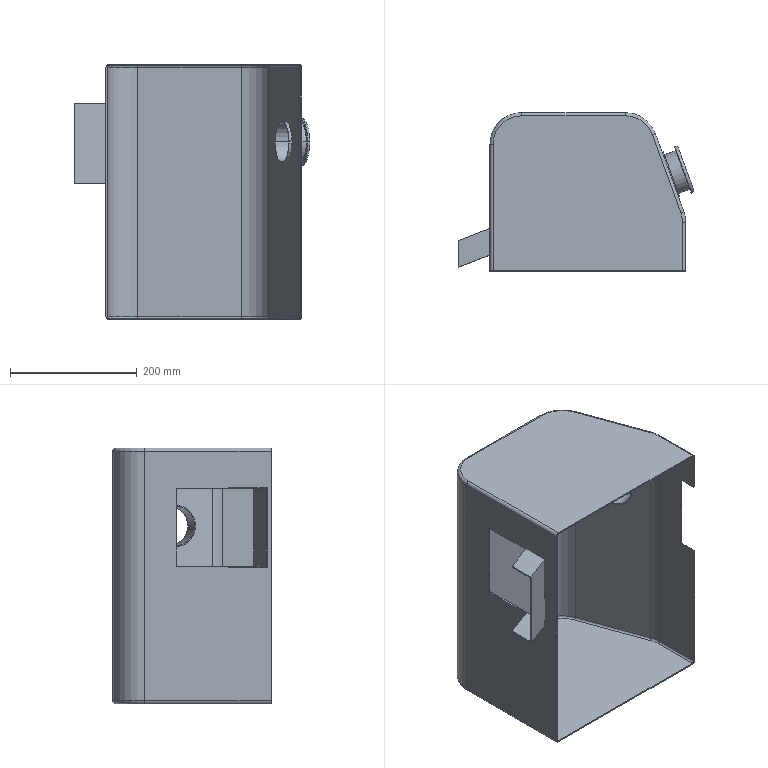Part | SolidWorks | features MoveFace 5, BaseBody 1 | 1 solid | 81 faces | box 371.669 x 250 x 404 mm | volume 855867 mm3 | plane 33 | cylinder 30 | torus 18 | commonest cylinder face diameters 6 x8 10 x8 65 x4 96 x3 100 x3 62 x2